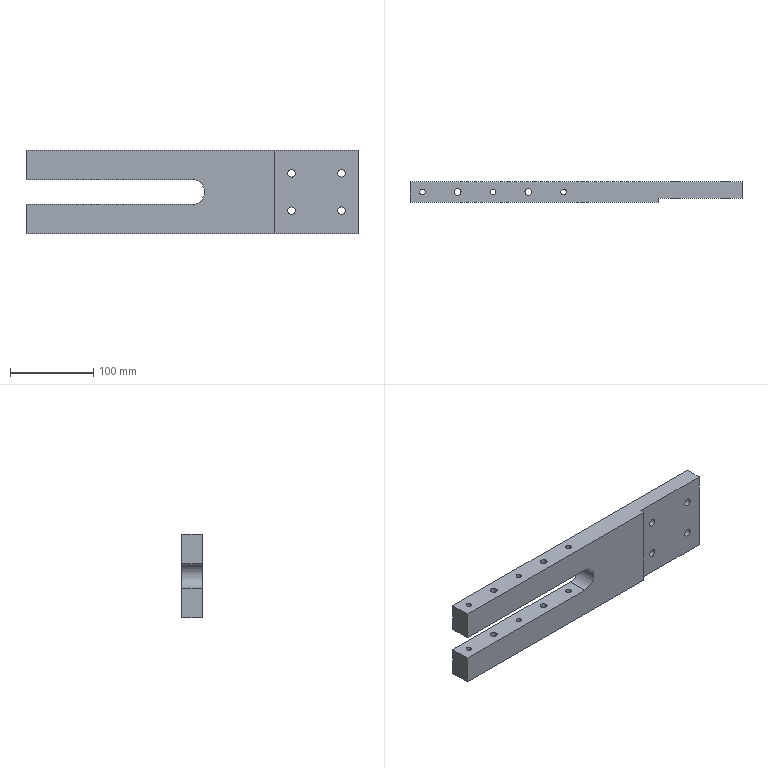Part | STEP file | SN10_001_001_PLACA | 1 solid | 30 faces | box 400 x 25 x 100 mm | volume 770318 mm3 | cylinder 17 | plane 11 | cone 2 | commonest cylinder face diameters 6.647 x8 8 x4 9 x4 30 x1